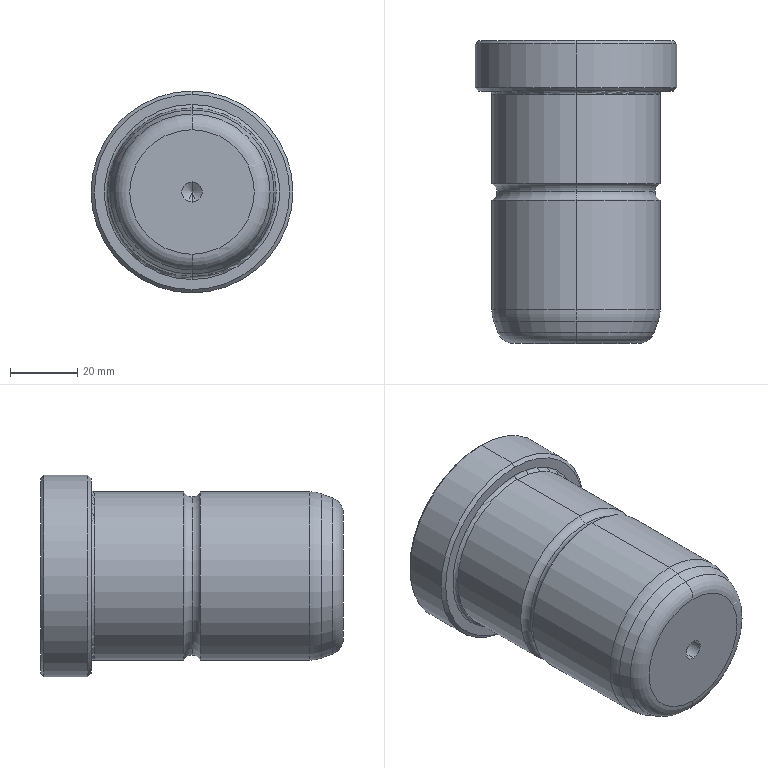Part | STEP file | Coluna fechamento - torre - 1 cav | 1 solid | 33 faces | box 60 x 90 x 60 mm | volume 186134 mm3 | torus 10 | cone 10 | cylinder 10 | plane 3 | commonest cylinder face diameters 6 x4 50 x4 60 x2